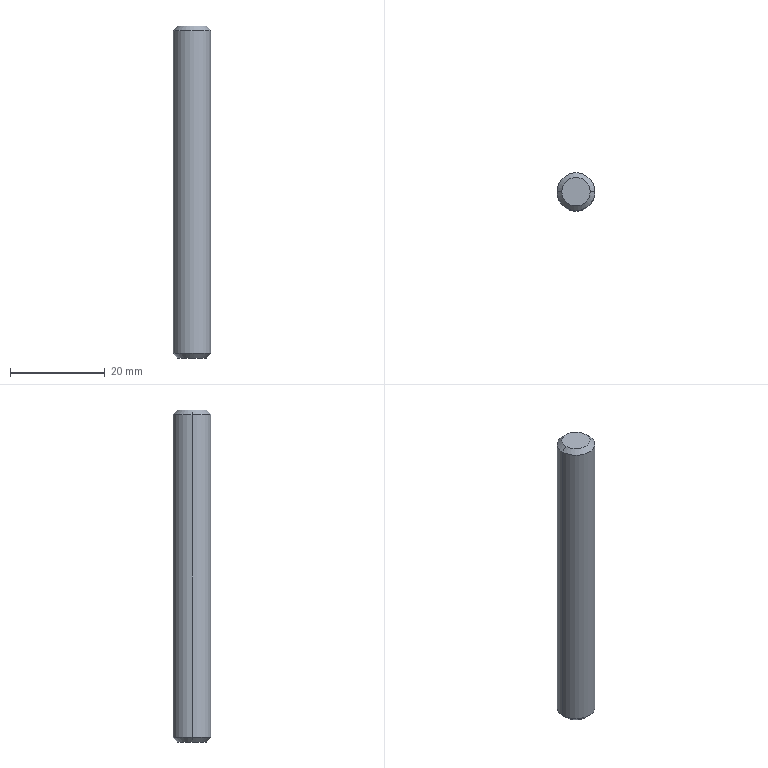Part | STEP file | CHOT DINH VI_2 | 1 solid | 8 faces | box 8 x 8 x 70 mm | volume 3496 mm3 | cone 4 | cylinder 2 | plane 2 | commonest cylinder face diameters 8 x2
STEP:
#1=CARTESIAN_POINT('',(0.,0.,0.));
#2=DIRECTION('',(0.,0.,1.));
#3=DIRECTION('',(1.,0.,0.));
#4=AXIS2_PLACEMENT_3D('',#1,#2,#3);
#5=CARTESIAN_POINT('',(4.,0.,1.));
#6=VERTEX_POINT('',#5);
#7=CARTESIAN_POINT('',(-4.,0.,1.));
#8=VERTEX_POINT('',#7);
#9=CARTESIAN_POINT('',(0.,0.,1.));
#10=DIRECTION('',(0.,0.,1.));
#11=DIRECTION('',(1.,0.,0.));
#12=AXIS2_PLACEMENT_3D('',#9,#10,#11);
#13=CIRCLE('',#12,4.);
#14=CARTESIAN_POINT('',(0.,0.,0.));
#15=DIRECTION('',(0.,0.,1.));
#16=DIRECTION('',(1.,0.,0.));
#17=AXIS2_PLACEMENT_3D('',#14,#15,#16);
#18=CYLINDRICAL_SURFACE('',#17,4.);
#19=CARTESIAN_POINT('',(0.,1.));
#20=DIRECTION('',(1.,0.));
#21=VECTOR('',#20,1.);
#22=LINE('',#19,#21);
#23=(GEOMETRIC_REPRESENTATION_CONTEXT(2)PARAMETRIC_REPRESENTATION_CONTEXT()REPRESENTATION_CONTEXT('',''));
#24=DEFINITIONAL_REPRESENTATION('',(#22),#23);
#25=PCURVE('',#18,#24);
#26=CARTESIAN_POINT('',(0.,0.,1.));
#27=DIRECTION('',(0.,0.,1.));
#28=DIRECTION('',(1.,0.,0.));
#29=AXIS2_PLACEMENT_3D('',#26,#27,#28);
#30=CONICAL_SURFACE('',#29,4.,0.7854);
#31=CARTESIAN_POINT('',(0.,0.));
#32=DIRECTION('',(1.,0.));
#33=VECTOR('',#32,1.);
#34=LINE('',#31,#33);
#35=(GEOMETRIC_REPRESENTATION_CONTEXT(2)PARAMETRIC_REPRESENTATION_CONTEXT()REPRESENTATION_CONTEXT('',''));
#36=DEFINITIONAL_REPRESENTATION('',(#34),#35);
#37=PCURVE('',#30,#36);
#38=SURFACE_CURVE('',#13,(#25,#37),.PCURVE_S1.);
#39=EDGE_CURVE('',#6,#8,#38,.T.);
#40=ORIENTED_EDGE('',*,*,#39,.T.);
#41=CARTESIAN_POINT('',(-4.,0.,69.));
#42=VERTEX_POINT('',#41);
#43=CARTESIAN_POINT('',(-4.,0.,0.));
#44=DIRECTION('',(0.,0.,1.));
#45=VECTOR('',#44,1.);
#46=LINE('',#43,#45);
#47=CARTESIAN_POINT('',(3.142,0.));
#48=DIRECTION('',(0.,1.));
#49=VECTOR('',#48,1.);
#50=LINE('',#47,#49);
#51=(GEOMETRIC_REPRESENTATION_CONTEXT(2)PARAMETRIC_REPRESENTATION_CONTEXT()REPRESENTATION_CONTEXT('',''));
#52=DEFINITIONAL_REPRESENTATION('',(#50),#51);
#53=PCURVE('',#18,#52);
#54=CARTESIAN_POINT('',(0.,0.,0.));
#55=DIRECTION('',(0.,0.,1.));
#56=DIRECTION('',(1.,0.,0.));
#57=AXIS2_PLACEMENT_3D('',#54,#55,#56);
#58=CYLINDRICAL_SURFACE('',#57,4.);
#59=CARTESIAN_POINT('',(3.142,0.));
#60=DIRECTION('',(0.,1.));
#61=VECTOR('',#60,1.);
#62=LINE('',#59,#61);
#63=(GEOMETRIC_REPRESENTATION_CONTEXT(2)PARAMETRIC_REPRESENTATION_CONTEXT()REPRESENTATION_CONTEXT('',''));
#64=DEFINITIONAL_REPRESENTATION('',(#62),#63);
#65=PCURVE('',#58,#64);
#66=SURFACE_CURVE('',#46,(#53,#65),.PCURVE_S1.);
#67=EDGE_CURVE('',#8,#42,#66,.T.);
#68=ORIENTED_EDGE('',*,*,#67,.T.);
#69=CARTESIAN_POINT('',(4.,0.,69.));
#70=VERTEX_POINT('',#69);
#71=CARTESIAN_POINT('',(0.,0.,69.));
#72=DIRECTION('',(0.,0.,-1.));
#73=DIRECTION('',(1.,0.,0.));
#74=AXIS2_PLACEMENT_3D('',#71,#72,#73);
#75=CIRCLE('',#74,4.);
#76=CARTESIAN_POINT('',(6.283,69.));
#77=DIRECTION('',(-1.,0.));
#78=VECTOR('',#77,1.);
#79=LINE('',#76,#78);
#80=(GEOMETRIC_REPRESENTATION_CONTEXT(2)PARAMETRIC_REPRESENTATION_CONTEXT()REPRESENTATION_CONTEXT('',''));
#81=DEFINITIONAL_REPRESENTATION('',(#79),#80);
#82=PCURVE('',#18,#81);
#83=CARTESIAN_POINT('',(0.,0.,69.));
#84=DIRECTION('',(0.,0.,-1.));
#85=DIRECTION('',(-1.,0.,0.));
#86=AXIS2_PLACEMENT_3D('',#83,#84,#85);
#87=CONICAL_SURFACE('',#86,4.,0.7854);
#88=CARTESIAN_POINT('',(-3.142,0.));
#89=DIRECTION('',(1.,0.));
#90=VECTOR('',#89,1.);
#91=LINE('',#88,#90);
#92=(GEOMETRIC_REPRESENTATION_CONTEXT(2)PARAMETRIC_REPRESENTATION_CONTEXT()REPRESENTATION_CONTEXT('',''));
#93=DEFINITIONAL_REPRESENTATION('',(#91),#92);
#94=PCURVE('',#87,#93);
#95=SURFACE_CURVE('',#75,(#82,#94),.PCURVE_S1.);
#96=EDGE_CURVE('',#42,#70,#95,.T.);
#97=ORIENTED_EDGE('',*,*,#96,.T.);
#98=CARTESIAN_POINT('',(4.,0.,0.));
#99=DIRECTION('',(0.,0.,1.));
#100=VECTOR('',#99,1.);
#101=LINE('',#98,#100);
#102=CARTESIAN_POINT('',(0.,0.));
#103=DIRECTION('',(0.,1.));
#104=VECTOR('',#103,1.);
#105=LINE('',#102,#104);
#106=(GEOMETRIC_REPRESENTATION_CONTEXT(2)PARAMETRIC_REPRESENTATION_CONTEXT()REPRESENTATION_CONTEXT('',''));
#107=DEFINITIONAL_REPRESENTATION('',(#105),#106);
#108=PCURVE('',#18,#107);
#109=CARTESIAN_POINT('',(6.283,0.));
#110=DIRECTION('',(0.,1.));
#111=VECTOR('',#110,1.);
#112=LINE('',#109,#111);
#113=(GEOMETRIC_REPRESENTATION_CONTEXT(2)PARAMETRIC_REPRESENTATION_CONTEXT()REPRESENTATION_CONTEXT('',''));
#114=DEFINITIONAL_REPRESENTATION('',(#112),#113);
#115=PCURVE('',#58,#114);
#116=SURFACE_CURVE('',#101,(#108,#115),.PCURVE_S1.);
#117=EDGE_CURVE('',#6,#70,#116,.T.);
#118=ORIENTED_EDGE('',*,*,#117,.F.);
#119=EDGE_LOOP('',(#40,#68,#97,#118));
#120=FACE_BOUND('',#119,.T.);
#121=ADVANCED_FACE('',(#120),#18,.T.);
#122=CARTESIAN_POINT('',(3.,0.,0.));
#123=VERTEX_POINT('',#122);
#124=CARTESIAN_POINT('',(-3.,0.,0.));
#125=VERTEX_POINT('',#124);
#126=CARTESIAN_POINT('',(0.,0.,0.));
#127=DIRECTION('',(0.,0.,1.));
#128=DIRECTION('',(1.,0.,0.));
#129=AXIS2_PLACEMENT_3D('',#126,#127,#128);
#130=CIRCLE('',#129,3.);
#131=CARTESIAN_POINT('',(0.,-1.));
#132=DIRECTION('',(1.,0.));
#133=VECTOR('',#132,1.);
#134=LINE('',#131,#133);
#135=(GEOMETRIC_REPRESENTATION_CONTEXT(2)PARAMETRIC_REPRESENTATION_CONTEXT()REPRESENTATION_CONTEXT('',''));
#136=DEFINITIONAL_REPRESENTATION('',(#134),#135);
#137=PCURVE('',#30,#136);
#138=CARTESIAN_POINT('',(0.,0.,0.));
#139=DIRECTION('',(0.,0.,-1.));
#140=DIRECTION('',(-1.,0.,0.));
#141=AXIS2_PLACEMENT_3D('',#138,#139,#140);
#142=PLANE('',#141);
#143=CARTESIAN_POINT('',(-3.,0.));
#144=CARTESIAN_POINT('',(-3.,5.196));
#145=CARTESIAN_POINT('',(1.5,2.598));
#146=CARTESIAN_POINT('',(6.,0.));
#147=CARTESIAN_POINT('',(1.5,-2.598));
#148=CARTESIAN_POINT('',(-3.,-5.196));
#149=CARTESIAN_POINT('',(-3.,0.));
#150=(BOUNDED_CURVE()B_SPLINE_CURVE(2,(#143,#144,#145,#146,#147,#148,#149),.UNSPECIFIED.,.T.,.F.)B_SPLINE_CURVE_WITH_KNOTS((1,2,2,2,2,1),(-2.094,0.,2.094,4.189,6.283,8.378),.UNSPECIFIED.)CURVE()GEOMETRIC_REPRESENTATION_ITEM()RATIONAL_B_SPLINE_CURVE((1.,0.5,1.,0.5,1.,0.5,1.))REPRESENTATION_ITEM(''));
#151=(GEOMETRIC_REPRESENTATION_CONTEXT(2)PARAMETRIC_REPRESENTATION_CONTEXT()REPRESENTATION_CONTEXT('',''));
#152=DEFINITIONAL_REPRESENTATION('',(#150),#151);
#153=PCURVE('',#142,#152);
#154=SURFACE_CURVE('',#130,(#137,#153),.PCURVE_S1.);
#155=EDGE_CURVE('',#123,#125,#154,.T.);
#156=ORIENTED_EDGE('',*,*,#155,.T.);
#157=CARTESIAN_POINT('',(-4.,0.,1.));
#158=DIRECTION('',(-0.7071,0.,0.7071));
#159=VECTOR('',#158,1.);
#160=LINE('',#157,#159);
#161=CARTESIAN_POINT('',(3.142,0.));
#162=DIRECTION('',(0.,1.));
#163=VECTOR('',#162,1.);
#164=LINE('',#161,#163);
#165=(GEOMETRIC_REPRESENTATION_CONTEXT(2)PARAMETRIC_REPRESENTATION_CONTEXT()REPRESENTATION_CONTEXT('',''));
#166=DEFINITIONAL_REPRESENTATION('',(#164),#165);
#167=PCURVE('',#30,#166);
#168=CARTESIAN_POINT('',(0.,0.,1.));
#169=DIRECTION('',(0.,0.,1.));
#170=DIRECTION('',(1.,0.,0.));
#171=AXIS2_PLACEMENT_3D('',#168,#169,#170);
#172=CONICAL_SURFACE('',#171,4.,0.7854);
#173=CARTESIAN_POINT('',(3.142,0.));
#174=DIRECTION('',(0.,1.));
#175=VECTOR('',#174,1.);
#176=LINE('',#173,#175);
#177=(GEOMETRIC_REPRESENTATION_CONTEXT(2)PARAMETRIC_REPRESENTATION_CONTEXT()REPRESENTATION_CONTEXT('',''));
#178=DEFINITIONAL_REPRESENTATION('',(#176),#177);
#179=PCURVE('',#172,#178);
#180=SURFACE_CURVE('',#160,(#167,#179),.PCURVE_S1.);
#181=EDGE_CURVE('',#125,#8,#180,.T.);
#182=ORIENTED_EDGE('',*,*,#181,.T.);
#183=ORIENTED_EDGE('',*,*,#39,.F.);
#184=CARTESIAN_POINT('',(4.,0.,1.));
#185=DIRECTION('',(0.7071,0.,0.7071));
#186=VECTOR('',#185,1.);
#187=LINE('',#184,#186);
#188=CARTESIAN_POINT('',(0.,0.));
#189=DIRECTION('',(0.,1.));
#190=VECTOR('',#189,1.);
#191=LINE('',#188,#190);
#192=(GEOMETRIC_REPRESENTATION_CONTEXT(2)PARAMETRIC_REPRESENTATION_CONTEXT()REPRESENTATION_CONTEXT('',''));
#193=DEFINITIONAL_REPRESENTATION('',(#191),#192);
#194=PCURVE('',#30,#193);
#195=CARTESIAN_POINT('',(6.283,0.));
#196=DIRECTION('',(0.,1.));
#197=VECTOR('',#196,1.);
#198=LINE('',#195,#197);
#199=(GEOMETRIC_REPRESENTATION_CONTEXT(2)PARAMETRIC_REPRESENTATION_CONTEXT()REPRESENTATION_CONTEXT('',''));
#200=DEFINITIONAL_REPRESENTATION('',(#198),#199);
#201=PCURVE('',#172,#200);
#202=SURFACE_CURVE('',#187,(#194,#201),.PCURVE_S1.);
#203=EDGE_CURVE('',#123,#6,#202,.T.);
#204=ORIENTED_EDGE('',*,*,#203,.F.);
#205=EDGE_LOOP('',(#156,#182,#183,#204));
#206=FACE_BOUND('',#205,.T.);
#207=ADVANCED_FACE('',(#206),#30,.T.);
#208=CARTESIAN_POINT('',(-3.,0.,70.));
#209=VERTEX_POINT('',#208);
#210=CARTESIAN_POINT('',(3.,0.,70.));
#211=VERTEX_POINT('',#210);
#212=CARTESIAN_POINT('',(0.,0.,70.));
#213=DIRECTION('',(0.,0.,-1.));
#214=DIRECTION('',(-1.,0.,0.));
#215=AXIS2_PLACEMENT_3D('',#212,#213,#214);
#216=CIRCLE('',#215,3.);
#217=CARTESIAN_POINT('',(0.,-1.));
#218=DIRECTION('',(1.,0.));
#219=VECTOR('',#218,1.);
#220=LINE('',#217,#219);
#221=(GEOMETRIC_REPRESENTATION_CONTEXT(2)PARAMETRIC_REPRESENTATION_CONTEXT()REPRESENTATION_CONTEXT('',''));
#222=DEFINITIONAL_REPRESENTATION('',(#220),#221);
#223=PCURVE('',#87,#222);
#224=CARTESIAN_POINT('',(0.,0.,70.));
#225=DIRECTION('',(0.,0.,-1.));
#226=DIRECTION('',(-1.,0.,0.));
#227=AXIS2_PLACEMENT_3D('',#224,#225,#226);
#228=PLANE('',#227);
#229=CARTESIAN_POINT('',(0.,0.));
#230=DIRECTION('',(1.,0.));
#231=AXIS2_PLACEMENT_2D('',#229,#230);
#232=CIRCLE('',#231,3.);
#233=(GEOMETRIC_REPRESENTATION_CONTEXT(2)PARAMETRIC_REPRESENTATION_CONTEXT()REPRESENTATION_CONTEXT('',''));
#234=DEFINITIONAL_REPRESENTATION('',(#232),#233);
#235=PCURVE('',#228,#234);
#236=SURFACE_CURVE('',#216,(#223,#235),.PCURVE_S1.);
#237=EDGE_CURVE('',#209,#211,#236,.T.);
#238=ORIENTED_EDGE('',*,*,#237,.T.);
#239=CARTESIAN_POINT('',(4.,0.,69.));
#240=DIRECTION('',(0.7071,0.,-0.7071));
#241=VECTOR('',#240,1.);
#242=LINE('',#239,#241);
#243=CARTESIAN_POINT('',(3.142,0.));
#244=DIRECTION('',(0.,1.));
#245=VECTOR('',#244,1.);
#246=LINE('',#243,#245);
#247=(GEOMETRIC_REPRESENTATION_CONTEXT(2)PARAMETRIC_REPRESENTATION_CONTEXT()REPRESENTATION_CONTEXT('',''));
#248=DEFINITIONAL_REPRESENTATION('',(#246),#247);
#249=PCURVE('',#87,#248);
#250=CARTESIAN_POINT('',(0.,0.,69.));
#251=DIRECTION('',(0.,0.,-1.));
#252=DIRECTION('',(-1.,0.,0.));
#253=AXIS2_PLACEMENT_3D('',#250,#251,#252);
#254=CONICAL_SURFACE('',#253,4.,0.7854);
#255=CARTESIAN_POINT('',(3.142,0.));
#256=DIRECTION('',(0.,1.));
#257=VECTOR('',#256,1.);
#258=LINE('',#255,#257);
#259=(GEOMETRIC_REPRESENTATION_CONTEXT(2)PARAMETRIC_REPRESENTATION_CONTEXT()REPRESENTATION_CONTEXT('',''));
#260=DEFINITIONAL_REPRESENTATION('',(#258),#259);
#261=PCURVE('',#254,#260);
#262=SURFACE_CURVE('',#242,(#249,#261),.PCURVE_S1.);
#263=EDGE_CURVE('',#211,#70,#262,.T.);
#264=ORIENTED_EDGE('',*,*,#263,.T.);
#265=ORIENTED_EDGE('',*,*,#96,.F.);
#266=CARTESIAN_POINT('',(-4.,0.,69.));
#267=DIRECTION('',(-0.7071,0.,-0.7071));
#268=VECTOR('',#267,1.);
#269=LINE('',#266,#268);
#270=CARTESIAN_POINT('',(0.,0.));
#271=DIRECTION('',(0.,1.));
#272=VECTOR('',#271,1.);
#273=LINE('',#270,#272);
#274=(GEOMETRIC_REPRESENTATION_CONTEXT(2)PARAMETRIC_REPRESENTATION_CONTEXT()REPRESENTATION_CONTEXT('',''));
#275=DEFINITIONAL_REPRESENTATION('',(#273),#274);
#276=PCURVE('',#87,#275);
#277=CARTESIAN_POINT('',(6.283,0.));
#278=DIRECTION('',(0.,1.));
#279=VECTOR('',#278,1.);
#280=LINE('',#277,#279);
#281=(GEOMETRIC_REPRESENTATION_CONTEXT(2)PARAMETRIC_REPRESENTATION_CONTEXT()REPRESENTATION_CONTEXT('',''));
#282=DEFINITIONAL_REPRESENTATION('',(#280),#281);
#283=PCURVE('',#254,#282);
#284=SURFACE_CURVE('',#269,(#276,#283),.PCURVE_S1.);
#285=EDGE_CURVE('',#209,#42,#284,.T.);
#286=ORIENTED_EDGE('',*,*,#285,.F.);
#287=EDGE_LOOP('',(#238,#264,#265,#286));
#288=FACE_BOUND('',#287,.T.);
#289=ADVANCED_FACE('',(#288),#87,.T.);
#290=ORIENTED_EDGE('',*,*,#67,.F.);
#291=CARTESIAN_POINT('',(0.,0.,1.));
#292=DIRECTION('',(0.,0.,1.));
#293=DIRECTION('',(1.,0.,0.));
#294=AXIS2_PLACEMENT_3D('',#291,#292,#293);
#295=CIRCLE('',#294,4.);
#296=CARTESIAN_POINT('',(0.,1.));
#297=DIRECTION('',(1.,0.));
#298=VECTOR('',#297,1.);
#299=LINE('',#296,#298);
#300=(GEOMETRIC_REPRESENTATION_CONTEXT(2)PARAMETRIC_REPRESENTATION_CONTEXT()REPRESENTATION_CONTEXT('',''));
#301=DEFINITIONAL_REPRESENTATION('',(#299),#300);
#302=PCURVE('',#58,#301);
#303=CARTESIAN_POINT('',(0.,0.));
#304=DIRECTION('',(1.,0.));
#305=VECTOR('',#304,1.);
#306=LINE('',#303,#305);
#307=(GEOMETRIC_REPRESENTATION_CONTEXT(2)PARAMETRIC_REPRESENTATION_CONTEXT()REPRESENTATION_CONTEXT('',''));
#308=DEFINITIONAL_REPRESENTATION('',(#306),#307);
#309=PCURVE('',#172,#308);
#310=SURFACE_CURVE('',#295,(#302,#309),.PCURVE_S1.);
#311=EDGE_CURVE('',#8,#6,#310,.T.);
#312=ORIENTED_EDGE('',*,*,#311,.T.);
#313=ORIENTED_EDGE('',*,*,#117,.T.);
#314=CARTESIAN_POINT('',(0.,0.,69.));
#315=DIRECTION('',(0.,0.,-1.));
#316=DIRECTION('',(1.,0.,0.));
#317=AXIS2_PLACEMENT_3D('',#314,#315,#316);
#318=CIRCLE('',#317,4.);
#319=CARTESIAN_POINT('',(6.283,69.));
#320=DIRECTION('',(-1.,0.));
#321=VECTOR('',#320,1.);
#322=LINE('',#319,#321);
#323=(GEOMETRIC_REPRESENTATION_CONTEXT(2)PARAMETRIC_REPRESENTATION_CONTEXT()REPRESENTATION_CONTEXT('',''));
#324=DEFINITIONAL_REPRESENTATION('',(#322),#323);
#325=PCURVE('',#58,#324);
#326=CARTESIAN_POINT('',(3.142,0.));
#327=DIRECTION('',(1.,0.));
#328=VECTOR('',#327,1.);
#329=LINE('',#326,#328);
#330=(GEOMETRIC_REPRESENTATION_CONTEXT(2)PARAMETRIC_REPRESENTATION_CONTEXT()REPRESENTATION_CONTEXT('',''));
#331=DEFINITIONAL_REPRESENTATION('',(#329),#330);
#332=PCURVE('',#254,#331);
#333=SURFACE_CURVE('',#318,(#325,#332),.PCURVE_S1.);
#334=EDGE_CURVE('',#70,#42,#333,.T.);
#335=ORIENTED_EDGE('',*,*,#334,.T.);
#336=EDGE_LOOP('',(#290,#312,#313,#335));
#337=FACE_BOUND('',#336,.T.);
#338=ADVANCED_FACE('',(#337),#58,.T.);
#339=ORIENTED_EDGE('',*,*,#181,.F.);
#340=CARTESIAN_POINT('',(0.,0.,0.));
#341=DIRECTION('',(0.,0.,1.));
#342=DIRECTION('',(1.,0.,0.));
#343=AXIS2_PLACEMENT_3D('',#340,#341,#342);
#344=CIRCLE('',#343,3.);
#345=CARTESIAN_POINT('',(0.,-1.));
#346=DIRECTION('',(1.,0.));
#347=VECTOR('',#346,1.);
#348=LINE('',#345,#347);
#349=(GEOMETRIC_REPRESENTATION_CONTEXT(2)PARAMETRIC_REPRESENTATION_CONTEXT()REPRESENTATION_CONTEXT('',''));
#350=DEFINITIONAL_REPRESENTATION('',(#348),#349);
#351=PCURVE('',#172,#350);
#352=CARTESIAN_POINT('',(-3.,0.));
#353=CARTESIAN_POINT('',(-3.,5.196));
#354=CARTESIAN_POINT('',(1.5,2.598));
#355=CARTESIAN_POINT('',(6.,0.));
#356=CARTESIAN_POINT('',(1.5,-2.598));
#357=CARTESIAN_POINT('',(-3.,-5.196));
#358=CARTESIAN_POINT('',(-3.,0.));
#359=(BOUNDED_CURVE()B_SPLINE_CURVE(2,(#352,#353,#354,#355,#356,#357,#358),.UNSPECIFIED.,.T.,.F.)B_SPLINE_CURVE_WITH_KNOTS((1,2,2,2,2,1),(-2.094,0.,2.094,4.189,6.283,8.378),.UNSPECIFIED.)CURVE()GEOMETRIC_REPRESENTATION_ITEM()RATIONAL_B_SPLINE_CURVE((1.,0.5,1.,0.5,1.,0.5,1.))REPRESENTATION_ITEM(''));
#360=(GEOMETRIC_REPRESENTATION_CONTEXT(2)PARAMETRIC_REPRESENTATION_CONTEXT()REPRESENTATION_CONTEXT('',''));
#361=DEFINITIONAL_REPRESENTATION('',(#359),#360);
#362=PCURVE('',#142,#361);
#363=SURFACE_CURVE('',#344,(#351,#362),.PCURVE_S1.);
#364=EDGE_CURVE('',#125,#123,#363,.T.);
#365=ORIENTED_EDGE('',*,*,#364,.T.);
#366=ORIENTED_EDGE('',*,*,#203,.T.);
#367=ORIENTED_EDGE('',*,*,#311,.F.);
#368=EDGE_LOOP('',(#339,#365,#366,#367));
#369=FACE_BOUND('',#368,.T.);
#370=ADVANCED_FACE('',(#369),#172,.T.);
#371=ORIENTED_EDGE('',*,*,#263,.F.);
#372=CARTESIAN_POINT('',(0.,0.,70.));
#373=DIRECTION('',(0.,0.,-1.));
#374=DIRECTION('',(-1.,0.,0.));
#375=AXIS2_PLACEMENT_3D('',#372,#373,#374);
#376=CIRCLE('',#375,3.);
#377=CARTESIAN_POINT('',(0.,-1.));
#378=DIRECTION('',(1.,0.));
#379=VECTOR('',#378,1.);
#380=LINE('',#377,#379);
#381=(GEOMETRIC_REPRESENTATION_CONTEXT(2)PARAMETRIC_REPRESENTATION_CONTEXT()REPRESENTATION_CONTEXT('',''));
#382=DEFINITIONAL_REPRESENTATION('',(#380),#381);
#383=PCURVE('',#254,#382);
#384=CARTESIAN_POINT('',(0.,0.));
#385=DIRECTION('',(1.,0.));
#386=AXIS2_PLACEMENT_2D('',#384,#385);
#387=CIRCLE('',#386,3.);
#388=(GEOMETRIC_REPRESENTATION_CONTEXT(2)PARAMETRIC_REPRESENTATION_CONTEXT()REPRESENTATION_CONTEXT('',''));
#389=DEFINITIONAL_REPRESENTATION('',(#387),#388);
#390=PCURVE('',#228,#389);
#391=SURFACE_CURVE('',#376,(#383,#390),.PCURVE_S1.);
#392=EDGE_CURVE('',#211,#209,#391,.T.);
#393=ORIENTED_EDGE('',*,*,#392,.T.);
#394=ORIENTED_EDGE('',*,*,#285,.T.);
#395=ORIENTED_EDGE('',*,*,#334,.F.);
#396=EDGE_LOOP('',(#371,#393,#394,#395));
#397=FACE_BOUND('',#396,.T.);
#398=ADVANCED_FACE('',(#397),#254,.T.);
#399=ORIENTED_EDGE('',*,*,#155,.F.);
#400=ORIENTED_EDGE('',*,*,#364,.F.);
#401=EDGE_LOOP('',(#399,#400));
#402=FACE_BOUND('',#401,.T.);
#403=ADVANCED_FACE('',(#402),#142,.T.);
#404=ORIENTED_EDGE('',*,*,#237,.F.);
#405=ORIENTED_EDGE('',*,*,#392,.F.);
#406=EDGE_LOOP('',(#404,#405));
#407=FACE_BOUND('',#406,.T.);
#408=ADVANCED_FACE('',(#407),#228,.F.);
#409=CLOSED_SHELL('',(#121,#207,#289,#338,#370,#398,#403,#408));
#410=MANIFOLD_SOLID_BREP('',#409);
#411=(LENGTH_UNIT()NAMED_UNIT(*)SI_UNIT(.MILLI.,.METRE.));
#412=UNCERTAINTY_MEASURE_WITH_UNIT(LENGTH_MEASURE(0.0000001),#411,'','');
#413=(NAMED_UNIT(*)PLANE_ANGLE_UNIT()SI_UNIT($,.RADIAN.));
#414=(NAMED_UNIT(*)SI_UNIT($,.STERADIAN.)SOLID_ANGLE_UNIT());
#415=(GEOMETRIC_REPRESENTATION_CONTEXT(3)GLOBAL_UNCERTAINTY_ASSIGNED_CONTEXT((#412))GLOBAL_UNIT_ASSIGNED_CONTEXT((#411,#413,#414))REPRESENTATION_CONTEXT('',''));
#416=ADVANCED_BREP_SHAPE_REPRESENTATION('',(#4,#410),#415);